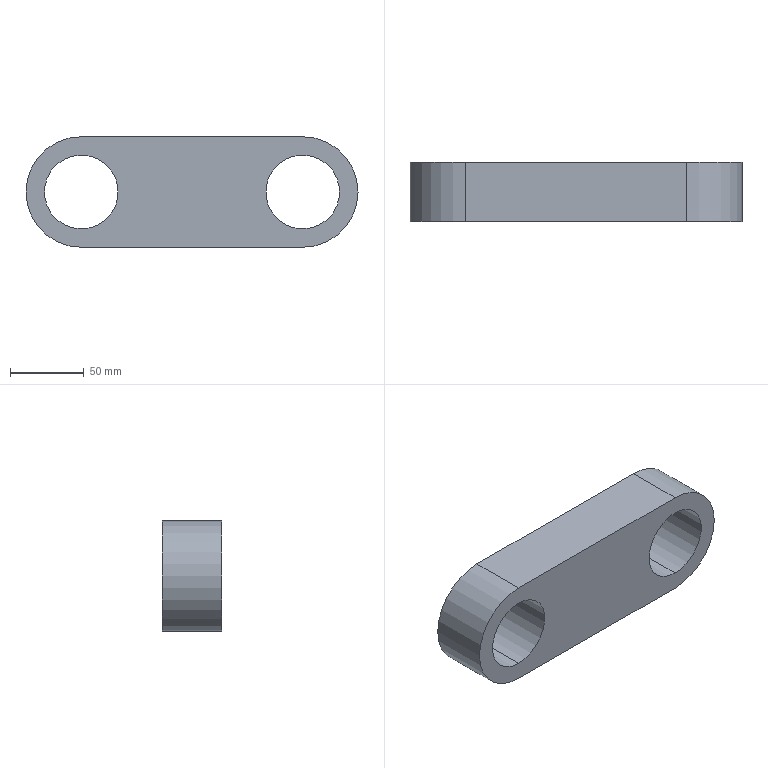Part | STEP file | LM-05-1240_default | 1 solid | 10 faces | box 225 x 40 x 75 mm | volume 469635 mm3 | cylinder 6 | plane 4 | commonest cylinder face diameters 50 x4 75 x2
STEP:
#1=CARTESIAN_POINT('',(0.,0.,0.));
#2=DIRECTION('',(0.,0.,1.));
#3=DIRECTION('',(1.,0.,0.));
#4=AXIS2_PLACEMENT_3D('',#1,#2,#3);
#5=CARTESIAN_POINT('',(75.,40.,-25.));
#6=VERTEX_POINT('',#5);
#7=CARTESIAN_POINT('',(75.,0.,-25.));
#8=VERTEX_POINT('',#7);
#9=CARTESIAN_POINT('',(75.,40.,-25.));
#10=DIRECTION('',(0.,-1.,0.));
#11=VECTOR('',#10,1.);
#12=LINE('',#9,#11);
#13=CARTESIAN_POINT('',(75.,40.,0.));
#14=DIRECTION('',(0.,-1.,0.));
#15=DIRECTION('',(0.,0.,-1.));
#16=AXIS2_PLACEMENT_3D('',#13,#14,#15);
#17=CYLINDRICAL_SURFACE('',#16,25.);
#18=CARTESIAN_POINT('',(6.283,0.));
#19=DIRECTION('',(0.,1.));
#20=VECTOR('',#19,1.);
#21=LINE('',#18,#20);
#22=(GEOMETRIC_REPRESENTATION_CONTEXT(2)PARAMETRIC_REPRESENTATION_CONTEXT()REPRESENTATION_CONTEXT('',''));
#23=DEFINITIONAL_REPRESENTATION('',(#21),#22);
#24=PCURVE('',#17,#23);
#25=CARTESIAN_POINT('',(75.,40.,0.));
#26=DIRECTION('',(0.,-1.,0.));
#27=DIRECTION('',(0.,0.,-1.));
#28=AXIS2_PLACEMENT_3D('',#25,#26,#27);
#29=CYLINDRICAL_SURFACE('',#28,25.);
#30=CARTESIAN_POINT('',(0.,0.));
#31=DIRECTION('',(0.,1.));
#32=VECTOR('',#31,1.);
#33=LINE('',#30,#32);
#34=(GEOMETRIC_REPRESENTATION_CONTEXT(2)PARAMETRIC_REPRESENTATION_CONTEXT()REPRESENTATION_CONTEXT('',''));
#35=DEFINITIONAL_REPRESENTATION('',(#33),#34);
#36=PCURVE('',#29,#35);
#37=SURFACE_CURVE('',#12,(#24,#36),.PCURVE_S1.);
#38=EDGE_CURVE('',#6,#8,#37,.T.);
#39=ORIENTED_EDGE('',*,*,#38,.T.);
#40=CARTESIAN_POINT('',(75.,0.,25.));
#41=VERTEX_POINT('',#40);
#42=CARTESIAN_POINT('',(75.,0.,0.));
#43=DIRECTION('',(0.,-1.,0.));
#44=DIRECTION('',(0.,0.,1.));
#45=AXIS2_PLACEMENT_3D('',#42,#43,#44);
#46=CIRCLE('',#45,25.);
#47=CARTESIAN_POINT('',(3.142,40.));
#48=DIRECTION('',(1.,0.));
#49=VECTOR('',#48,1.);
#50=LINE('',#47,#49);
#51=(GEOMETRIC_REPRESENTATION_CONTEXT(2)PARAMETRIC_REPRESENTATION_CONTEXT()REPRESENTATION_CONTEXT('',''));
#52=DEFINITIONAL_REPRESENTATION('',(#50),#51);
#53=PCURVE('',#17,#52);
#54=CARTESIAN_POINT('',(75.,0.,0.));
#55=DIRECTION('',(0.,-1.,0.));
#56=DIRECTION('',(0.,0.,-1.));
#57=AXIS2_PLACEMENT_3D('',#54,#55,#56);
#58=PLANE('',#57);
#59=CARTESIAN_POINT('',(0.,0.));
#60=DIRECTION('',(-1.,0.));
#61=AXIS2_PLACEMENT_2D('',#59,#60);
#62=CIRCLE('',#61,25.);
#63=(GEOMETRIC_REPRESENTATION_CONTEXT(2)PARAMETRIC_REPRESENTATION_CONTEXT()REPRESENTATION_CONTEXT('',''));
#64=DEFINITIONAL_REPRESENTATION('',(#62),#63);
#65=PCURVE('',#58,#64);
#66=SURFACE_CURVE('',#46,(#53,#65),.PCURVE_S1.);
#67=EDGE_CURVE('',#41,#8,#66,.T.);
#68=ORIENTED_EDGE('',*,*,#67,.F.);
#69=CARTESIAN_POINT('',(75.,40.,25.));
#70=VERTEX_POINT('',#69);
#71=CARTESIAN_POINT('',(75.,40.,25.));
#72=DIRECTION('',(0.,-1.,0.));
#73=VECTOR('',#72,1.);
#74=LINE('',#71,#73);
#75=CARTESIAN_POINT('',(3.142,0.));
#76=DIRECTION('',(0.,1.));
#77=VECTOR('',#76,1.);
#78=LINE('',#75,#77);
#79=(GEOMETRIC_REPRESENTATION_CONTEXT(2)PARAMETRIC_REPRESENTATION_CONTEXT()REPRESENTATION_CONTEXT('',''));
#80=DEFINITIONAL_REPRESENTATION('',(#78),#79);
#81=PCURVE('',#17,#80);
#82=CARTESIAN_POINT('',(3.142,0.));
#83=DIRECTION('',(0.,1.));
#84=VECTOR('',#83,1.);
#85=LINE('',#82,#84);
#86=(GEOMETRIC_REPRESENTATION_CONTEXT(2)PARAMETRIC_REPRESENTATION_CONTEXT()REPRESENTATION_CONTEXT('',''));
#87=DEFINITIONAL_REPRESENTATION('',(#85),#86);
#88=PCURVE('',#29,#87);
#89=SURFACE_CURVE('',#74,(#81,#88),.PCURVE_S1.);
#90=EDGE_CURVE('',#70,#41,#89,.T.);
#91=ORIENTED_EDGE('',*,*,#90,.F.);
#92=CARTESIAN_POINT('',(75.,40.,0.));
#93=DIRECTION('',(0.,-1.,0.));
#94=DIRECTION('',(0.,0.,1.));
#95=AXIS2_PLACEMENT_3D('',#92,#93,#94);
#96=CIRCLE('',#95,25.);
#97=CARTESIAN_POINT('',(3.142,0.));
#98=DIRECTION('',(1.,0.));
#99=VECTOR('',#98,1.);
#100=LINE('',#97,#99);
#101=(GEOMETRIC_REPRESENTATION_CONTEXT(2)PARAMETRIC_REPRESENTATION_CONTEXT()REPRESENTATION_CONTEXT('',''));
#102=DEFINITIONAL_REPRESENTATION('',(#100),#101);
#103=PCURVE('',#17,#102);
#104=CARTESIAN_POINT('',(75.,40.,0.));
#105=DIRECTION('',(0.,-1.,0.));
#106=DIRECTION('',(0.,0.,-1.));
#107=AXIS2_PLACEMENT_3D('',#104,#105,#106);
#108=PLANE('',#107);
#109=CARTESIAN_POINT('',(0.,0.));
#110=DIRECTION('',(-1.,0.));
#111=AXIS2_PLACEMENT_2D('',#109,#110);
#112=CIRCLE('',#111,25.);
#113=(GEOMETRIC_REPRESENTATION_CONTEXT(2)PARAMETRIC_REPRESENTATION_CONTEXT()REPRESENTATION_CONTEXT('',''));
#114=DEFINITIONAL_REPRESENTATION('',(#112),#113);
#115=PCURVE('',#108,#114);
#116=SURFACE_CURVE('',#96,(#103,#115),.PCURVE_S1.);
#117=EDGE_CURVE('',#70,#6,#116,.T.);
#118=ORIENTED_EDGE('',*,*,#117,.T.);
#119=EDGE_LOOP('',(#39,#68,#91,#118));
#120=FACE_BOUND('',#119,.F.);
#121=ADVANCED_FACE('',(#120),#17,.F.);
#122=CARTESIAN_POINT('',(-75.,40.,-25.));
#123=VERTEX_POINT('',#122);
#124=CARTESIAN_POINT('',(-75.,0.,-25.));
#125=VERTEX_POINT('',#124);
#126=CARTESIAN_POINT('',(-75.,40.,-25.));
#127=DIRECTION('',(0.,-1.,0.));
#128=VECTOR('',#127,1.);
#129=LINE('',#126,#128);
#130=CARTESIAN_POINT('',(-75.,40.,0.));
#131=DIRECTION('',(0.,-1.,0.));
#132=DIRECTION('',(0.,0.,-1.));
#133=AXIS2_PLACEMENT_3D('',#130,#131,#132);
#134=CYLINDRICAL_SURFACE('',#133,25.);
#135=CARTESIAN_POINT('',(6.283,0.));
#136=DIRECTION('',(0.,1.));
#137=VECTOR('',#136,1.);
#138=LINE('',#135,#137);
#139=(GEOMETRIC_REPRESENTATION_CONTEXT(2)PARAMETRIC_REPRESENTATION_CONTEXT()REPRESENTATION_CONTEXT('',''));
#140=DEFINITIONAL_REPRESENTATION('',(#138),#139);
#141=PCURVE('',#134,#140);
#142=CARTESIAN_POINT('',(-75.,40.,0.));
#143=DIRECTION('',(0.,-1.,0.));
#144=DIRECTION('',(0.,0.,-1.));
#145=AXIS2_PLACEMENT_3D('',#142,#143,#144);
#146=CYLINDRICAL_SURFACE('',#145,25.);
#147=CARTESIAN_POINT('',(0.,0.));
#148=DIRECTION('',(0.,1.));
#149=VECTOR('',#148,1.);
#150=LINE('',#147,#149);
#151=(GEOMETRIC_REPRESENTATION_CONTEXT(2)PARAMETRIC_REPRESENTATION_CONTEXT()REPRESENTATION_CONTEXT('',''));
#152=DEFINITIONAL_REPRESENTATION('',(#150),#151);
#153=PCURVE('',#146,#152);
#154=SURFACE_CURVE('',#129,(#141,#153),.PCURVE_S1.);
#155=EDGE_CURVE('',#123,#125,#154,.T.);
#156=ORIENTED_EDGE('',*,*,#155,.T.);
#157=CARTESIAN_POINT('',(-75.,0.,25.));
#158=VERTEX_POINT('',#157);
#159=CARTESIAN_POINT('',(-75.,0.,0.));
#160=DIRECTION('',(0.,-1.,0.));
#161=DIRECTION('',(0.,0.,1.));
#162=AXIS2_PLACEMENT_3D('',#159,#160,#161);
#163=CIRCLE('',#162,25.);
#164=CARTESIAN_POINT('',(3.142,40.));
#165=DIRECTION('',(1.,0.));
#166=VECTOR('',#165,1.);
#167=LINE('',#164,#166);
#168=(GEOMETRIC_REPRESENTATION_CONTEXT(2)PARAMETRIC_REPRESENTATION_CONTEXT()REPRESENTATION_CONTEXT('',''));
#169=DEFINITIONAL_REPRESENTATION('',(#167),#168);
#170=PCURVE('',#134,#169);
#171=CARTESIAN_POINT('',(0.,-150.));
#172=DIRECTION('',(-1.,0.));
#173=AXIS2_PLACEMENT_2D('',#171,#172);
#174=CIRCLE('',#173,25.);
#175=(GEOMETRIC_REPRESENTATION_CONTEXT(2)PARAMETRIC_REPRESENTATION_CONTEXT()REPRESENTATION_CONTEXT('',''));
#176=DEFINITIONAL_REPRESENTATION('',(#174),#175);
#177=PCURVE('',#58,#176);
#178=SURFACE_CURVE('',#163,(#170,#177),.PCURVE_S1.);
#179=EDGE_CURVE('',#158,#125,#178,.T.);
#180=ORIENTED_EDGE('',*,*,#179,.F.);
#181=CARTESIAN_POINT('',(-75.,40.,25.));
#182=VERTEX_POINT('',#181);
#183=CARTESIAN_POINT('',(-75.,40.,25.));
#184=DIRECTION('',(0.,-1.,0.));
#185=VECTOR('',#184,1.);
#186=LINE('',#183,#185);
#187=CARTESIAN_POINT('',(3.142,0.));
#188=DIRECTION('',(0.,1.));
#189=VECTOR('',#188,1.);
#190=LINE('',#187,#189);
#191=(GEOMETRIC_REPRESENTATION_CONTEXT(2)PARAMETRIC_REPRESENTATION_CONTEXT()REPRESENTATION_CONTEXT('',''));
#192=DEFINITIONAL_REPRESENTATION('',(#190),#191);
#193=PCURVE('',#134,#192);
#194=CARTESIAN_POINT('',(3.142,0.));
#195=DIRECTION('',(0.,1.));
#196=VECTOR('',#195,1.);
#197=LINE('',#194,#196);
#198=(GEOMETRIC_REPRESENTATION_CONTEXT(2)PARAMETRIC_REPRESENTATION_CONTEXT()REPRESENTATION_CONTEXT('',''));
#199=DEFINITIONAL_REPRESENTATION('',(#197),#198);
#200=PCURVE('',#146,#199);
#201=SURFACE_CURVE('',#186,(#193,#200),.PCURVE_S1.);
#202=EDGE_CURVE('',#182,#158,#201,.T.);
#203=ORIENTED_EDGE('',*,*,#202,.F.);
#204=CARTESIAN_POINT('',(-75.,40.,0.));
#205=DIRECTION('',(0.,-1.,0.));
#206=DIRECTION('',(0.,0.,1.));
#207=AXIS2_PLACEMENT_3D('',#204,#205,#206);
#208=CIRCLE('',#207,25.);
#209=CARTESIAN_POINT('',(3.142,0.));
#210=DIRECTION('',(1.,0.));
#211=VECTOR('',#210,1.);
#212=LINE('',#209,#211);
#213=(GEOMETRIC_REPRESENTATION_CONTEXT(2)PARAMETRIC_REPRESENTATION_CONTEXT()REPRESENTATION_CONTEXT('',''));
#214=DEFINITIONAL_REPRESENTATION('',(#212),#213);
#215=PCURVE('',#134,#214);
#216=CARTESIAN_POINT('',(0.,-150.));
#217=DIRECTION('',(-1.,0.));
#218=AXIS2_PLACEMENT_2D('',#216,#217);
#219=CIRCLE('',#218,25.);
#220=(GEOMETRIC_REPRESENTATION_CONTEXT(2)PARAMETRIC_REPRESENTATION_CONTEXT()REPRESENTATION_CONTEXT('',''));
#221=DEFINITIONAL_REPRESENTATION('',(#219),#220);
#222=PCURVE('',#108,#221);
#223=SURFACE_CURVE('',#208,(#215,#222),.PCURVE_S1.);
#224=EDGE_CURVE('',#182,#123,#223,.T.);
#225=ORIENTED_EDGE('',*,*,#224,.T.);
#226=EDGE_LOOP('',(#156,#180,#203,#225));
#227=FACE_BOUND('',#226,.F.);
#228=ADVANCED_FACE('',(#227),#134,.F.);
#229=CARTESIAN_POINT('',(75.,0.,-37.5));
#230=VERTEX_POINT('',#229);
#231=CARTESIAN_POINT('',(75.,0.,37.5));
#232=VERTEX_POINT('',#231);
#233=CARTESIAN_POINT('',(75.,0.,0.));
#234=DIRECTION('',(0.,-1.,0.));
#235=DIRECTION('',(0.,0.,-1.));
#236=AXIS2_PLACEMENT_3D('',#233,#234,#235);
#237=CIRCLE('',#236,37.5);
#238=CARTESIAN_POINT('',(75.,40.,0.));
#239=DIRECTION('',(0.,-1.,0.));
#240=DIRECTION('',(0.,0.,-1.));
#241=AXIS2_PLACEMENT_3D('',#238,#239,#240);
#242=CYLINDRICAL_SURFACE('',#241,37.5);
#243=CARTESIAN_POINT('',(0.,40.));
#244=DIRECTION('',(1.,0.));
#245=VECTOR('',#244,1.);
#246=LINE('',#243,#245);
#247=(GEOMETRIC_REPRESENTATION_CONTEXT(2)PARAMETRIC_REPRESENTATION_CONTEXT()REPRESENTATION_CONTEXT('',''));
#248=DEFINITIONAL_REPRESENTATION('',(#246),#247);
#249=PCURVE('',#242,#248);
#250=CARTESIAN_POINT('',(0.,0.));
#251=DIRECTION('',(1.,0.));
#252=AXIS2_PLACEMENT_2D('',#250,#251);
#253=CIRCLE('',#252,37.5);
#254=(GEOMETRIC_REPRESENTATION_CONTEXT(2)PARAMETRIC_REPRESENTATION_CONTEXT()REPRESENTATION_CONTEXT('',''));
#255=DEFINITIONAL_REPRESENTATION('',(#253),#254);
#256=PCURVE('',#58,#255);
#257=SURFACE_CURVE('',#237,(#249,#256),.PCURVE_S1.);
#258=EDGE_CURVE('',#230,#232,#257,.T.);
#259=ORIENTED_EDGE('',*,*,#258,.F.);
#260=CARTESIAN_POINT('',(75.,40.,-37.5));
#261=VERTEX_POINT('',#260);
#262=CARTESIAN_POINT('',(75.,40.,-37.5));
#263=DIRECTION('',(0.,-1.,0.));
#264=VECTOR('',#263,1.);
#265=LINE('',#262,#264);
#266=CARTESIAN_POINT('',(0.,0.));
#267=DIRECTION('',(0.,1.));
#268=VECTOR('',#267,1.);
#269=LINE('',#266,#268);
#270=(GEOMETRIC_REPRESENTATION_CONTEXT(2)PARAMETRIC_REPRESENTATION_CONTEXT()REPRESENTATION_CONTEXT('',''));
#271=DEFINITIONAL_REPRESENTATION('',(#269),#270);
#272=PCURVE('',#242,#271);
#273=CARTESIAN_POINT('',(-75.,40.,-37.5));
#274=DIRECTION('',(0.,0.,-1.));
#275=DIRECTION('',(-1.,0.,0.));
#276=AXIS2_PLACEMENT_3D('',#273,#274,#275);
#277=PLANE('',#276);
#278=CARTESIAN_POINT('',(-150.,0.));
#279=DIRECTION('',(0.,-1.));
#280=VECTOR('',#279,1.);
#281=LINE('',#278,#280);
#282=(GEOMETRIC_REPRESENTATION_CONTEXT(2)PARAMETRIC_REPRESENTATION_CONTEXT()REPRESENTATION_CONTEXT('',''));
#283=DEFINITIONAL_REPRESENTATION('',(#281),#282);
#284=PCURVE('',#277,#283);
#285=SURFACE_CURVE('',#265,(#272,#284),.PCURVE_S1.);
#286=EDGE_CURVE('',#261,#230,#285,.T.);
#287=ORIENTED_EDGE('',*,*,#286,.F.);
#288=CARTESIAN_POINT('',(75.,40.,37.5));
#289=VERTEX_POINT('',#288);
#290=CARTESIAN_POINT('',(75.,40.,0.));
#291=DIRECTION('',(0.,-1.,0.));
#292=DIRECTION('',(0.,0.,-1.));
#293=AXIS2_PLACEMENT_3D('',#290,#291,#292);
#294=CIRCLE('',#293,37.5);
#295=CARTESIAN_POINT('',(0.,0.));
#296=DIRECTION('',(1.,0.));
#297=VECTOR('',#296,1.);
#298=LINE('',#295,#297);
#299=(GEOMETRIC_REPRESENTATION_CONTEXT(2)PARAMETRIC_REPRESENTATION_CONTEXT()REPRESENTATION_CONTEXT('',''));
#300=DEFINITIONAL_REPRESENTATION('',(#298),#299);
#301=PCURVE('',#242,#300);
#302=CARTESIAN_POINT('',(0.,0.));
#303=DIRECTION('',(1.,0.));
#304=AXIS2_PLACEMENT_2D('',#302,#303);
#305=CIRCLE('',#304,37.5);
#306=(GEOMETRIC_REPRESENTATION_CONTEXT(2)PARAMETRIC_REPRESENTATION_CONTEXT()REPRESENTATION_CONTEXT('',''));
#307=DEFINITIONAL_REPRESENTATION('',(#305),#306);
#308=PCURVE('',#108,#307);
#309=SURFACE_CURVE('',#294,(#301,#308),.PCURVE_S1.);
#310=EDGE_CURVE('',#261,#289,#309,.T.);
#311=ORIENTED_EDGE('',*,*,#310,.T.);
#312=CARTESIAN_POINT('',(75.,40.,37.5));
#313=DIRECTION('',(0.,-1.,0.));
#314=VECTOR('',#313,1.);
#315=LINE('',#312,#314);
#316=CARTESIAN_POINT('',(3.142,0.));
#317=DIRECTION('',(0.,1.));
#318=VECTOR('',#317,1.);
#319=LINE('',#316,#318);
#320=(GEOMETRIC_REPRESENTATION_CONTEXT(2)PARAMETRIC_REPRESENTATION_CONTEXT()REPRESENTATION_CONTEXT('',''));
#321=DEFINITIONAL_REPRESENTATION('',(#319),#320);
#322=PCURVE('',#242,#321);
#323=CARTESIAN_POINT('',(75.,40.,37.5));
#324=DIRECTION('',(0.,0.,1.));
#325=DIRECTION('',(1.,0.,0.));
#326=AXIS2_PLACEMENT_3D('',#323,#324,#325);
#327=PLANE('',#326);
#328=CARTESIAN_POINT('',(0.,0.));
#329=DIRECTION('',(0.,-1.));
#330=VECTOR('',#329,1.);
#331=LINE('',#328,#330);
#332=(GEOMETRIC_REPRESENTATION_CONTEXT(2)PARAMETRIC_REPRESENTATION_CONTEXT()REPRESENTATION_CONTEXT('',''));
#333=DEFINITIONAL_REPRESENTATION('',(#331),#332);
#334=PCURVE('',#327,#333);
#335=SURFACE_CURVE('',#315,(#322,#334),.PCURVE_S1.);
#336=EDGE_CURVE('',#289,#232,#335,.T.);
#337=ORIENTED_EDGE('',*,*,#336,.T.);
#338=EDGE_LOOP('',(#259,#287,#311,#337));
#339=FACE_BOUND('',#338,.T.);
#340=ADVANCED_FACE('',(#339),#242,.T.);
#341=CARTESIAN_POINT('',(-75.,0.,-37.5));
#342=VERTEX_POINT('',#341);
#343=CARTESIAN_POINT('',(-75.,0.,-37.5));
#344=DIRECTION('',(1.,0.,0.));
#345=VECTOR('',#344,1.);
#346=LINE('',#343,#345);
#347=CARTESIAN_POINT('',(0.,-40.));
#348=DIRECTION('',(-1.,0.));
#349=VECTOR('',#348,1.);
#350=LINE('',#347,#349);
#351=(GEOMETRIC_REPRESENTATION_CONTEXT(2)PARAMETRIC_REPRESENTATION_CONTEXT()REPRESENTATION_CONTEXT('',''));
#352=DEFINITIONAL_REPRESENTATION('',(#350),#351);
#353=PCURVE('',#277,#352);
#354=CARTESIAN_POINT('',(37.5,-150.));
#355=DIRECTION('',(0.,1.));
#356=VECTOR('',#355,1.);
#357=LINE('',#354,#356);
#358=(GEOMETRIC_REPRESENTATION_CONTEXT(2)PARAMETRIC_REPRESENTATION_CONTEXT()REPRESENTATION_CONTEXT('',''));
#359=DEFINITIONAL_REPRESENTATION('',(#357),#358);
#360=PCURVE('',#58,#359);
#361=SURFACE_CURVE('',#346,(#353,#360),.PCURVE_S1.);
#362=EDGE_CURVE('',#342,#230,#361,.T.);
#363=ORIENTED_EDGE('',*,*,#362,.F.);
#364=CARTESIAN_POINT('',(-75.,40.,-37.5));
#365=VERTEX_POINT('',#364);
#366=CARTESIAN_POINT('',(-75.,40.,-37.5));
#367=DIRECTION('',(0.,-1.,0.));
#368=VECTOR('',#367,1.);
#369=LINE('',#366,#368);
#370=CARTESIAN_POINT('',(0.,0.));
#371=DIRECTION('',(0.,-1.));
#372=VECTOR('',#371,1.);
#373=LINE('',#370,#372);
#374=(GEOMETRIC_REPRESENTATION_CONTEXT(2)PARAMETRIC_REPRESENTATION_CONTEXT()REPRESENTATION_CONTEXT('',''));
#375=DEFINITIONAL_REPRESENTATION('',(#373),#374);
#376=PCURVE('',#277,#375);
#377=CARTESIAN_POINT('',(-75.,40.,0.));
#378=DIRECTION('',(0.,-1.,0.));
#379=DIRECTION('',(0.,0.,-1.));
#380=AXIS2_PLACEMENT_3D('',#377,#378,#379);
#381=CYLINDRICAL_SURFACE('',#380,37.5);
#382=CARTESIAN_POINT('',(6.283,0.));
#383=DIRECTION('',(0.,1.));
#384=VECTOR('',#383,1.);
#385=LINE('',#382,#384);
#386=(GEOMETRIC_REPRESENTATION_CONTEXT(2)PARAMETRIC_REPRESENTATION_CONTEXT()REPRESENTATION_CONTEXT('',''));
#387=DEFINITIONAL_REPRESENTATION('',(#385),#386);
#388=PCURVE('',#381,#387);
#389=SURFACE_CURVE('',#369,(#376,#388),.PCURVE_S1.);
#390=EDGE_CURVE('',#365,#342,#389,.T.);
#391=ORIENTED_EDGE('',*,*,#390,.F.);
#392=CARTESIAN_POINT('',(-75.,40.,-37.5));
#393=DIRECTION('',(1.,0.,0.));
#394=VECTOR('',#393,1.);
#395=LINE('',#392,#394);
#396=CARTESIAN_POINT('',(0.,0.));
#397=DIRECTION('',(-1.,0.));
#398=VECTOR('',#397,1.);
#399=LINE('',#396,#398);
#400=(GEOMETRIC_REPRESENTATION_CONTEXT(2)PARAMETRIC_REPRESENTATION_CONTEXT()REPRESENTATION_CONTEXT('',''));
#401=DEFINITIONAL_REPRESENTATION('',(#399),#400);
#402=PCURVE('',#277,#401);
#403=CARTESIAN_POINT('',(37.5,-150.));
#404=DIRECTION('',(0.,1.));
#405=VECTOR('',#404,1.);
#406=LINE('',#403,#405);
#407=(GEOMETRIC_REPRESENTATION_CONTEXT(2)PARAMETRIC_REPRESENTATION_CONTEXT()REPRESENTATION_CONTEXT('',''));
#408=DEFINITIONAL_REPRESENTATION('',(#406),#407);
#409=PCURVE('',#108,#408);
#410=SURFACE_CURVE('',#395,(#402,#409),.PCURVE_S1.);
#411=EDGE_CURVE('',#365,#261,#410,.T.);
#412=ORIENTED_EDGE('',*,*,#411,.T.);
#413=ORIENTED_EDGE('',*,*,#286,.T.);
#414=EDGE_LOOP('',(#363,#391,#412,#413));
#415=FACE_BOUND('',#414,.T.);
#416=ADVANCED_FACE('',(#415),#277,.T.);
#417=CARTESIAN_POINT('',(-75.,0.,37.5));
#418=VERTEX_POINT('',#417);
#419=CARTESIAN_POINT('',(-75.,0.,0.));
#420=DIRECTION('',(0.,-1.,0.));
#421=DIRECTION('',(0.,0.,-1.));
#422=AXIS2_PLACEMENT_3D('',#419,#420,#421);
#423=CIRCLE('',#422,37.5);
#424=CARTESIAN_POINT('',(0.,40.));
#425=DIRECTION('',(1.,0.));
#426=VECTOR('',#425,1.);
#427=LINE('',#424,#426);
#428=(GEOMETRIC_REPRESENTATION_CONTEXT(2)PARAMETRIC_REPRESENTATION_CONTEXT()REPRESENTATION_CONTEXT('',''));
#429=DEFINITIONAL_REPRESENTATION('',(#427),#428);
#430=PCURVE('',#381,#429);
#431=CARTESIAN_POINT('',(0.,-150.));
#432=DIRECTION('',(1.,0.));
#433=AXIS2_PLACEMENT_2D('',#431,#432);
#434=CIRCLE('',#433,37.5);
#435=(GEOMETRIC_REPRESENTATION_CONTEXT(2)PARAMETRIC_REPRESENTATION_CONTEXT()REPRESENTATION_CONTEXT('',''));
#436=DEFINITIONAL_REPRESENTATION('',(#434),#435);
#437=PCURVE('',#58,#436);
#438=SURFACE_CURVE('',#423,(#430,#437),.PCURVE_S1.);
#439=EDGE_CURVE('',#418,#342,#438,.T.);
#440=ORIENTED_EDGE('',*,*,#439,.F.);
#441=CARTESIAN_POINT('',(-75.,40.,37.5));
#442=VERTEX_POINT('',#441);
#443=CARTESIAN_POINT('',(-75.,40.,37.5));
#444=DIRECTION('',(0.,-1.,0.));
#445=VECTOR('',#444,1.);
#446=LINE('',#443,#445);
#447=CARTESIAN_POINT('',(3.142,0.));
#448=DIRECTION('',(0.,1.));
#449=VECTOR('',#448,1.);
#450=LINE('',#447,#449);
#451=(GEOMETRIC_REPRESENTATION_CONTEXT(2)PARAMETRIC_REPRESENTATION_CONTEXT()REPRESENTATION_CONTEXT('',''));
#452=DEFINITIONAL_REPRESENTATION('',(#450),#451);
#453=PCURVE('',#381,#452);
#454=CARTESIAN_POINT('',(-150.,0.));
#455=DIRECTION('',(0.,-1.));
#456=VECTOR('',#455,1.);
#457=LINE('',#454,#456);
#458=(GEOMETRIC_REPRESENTATION_CONTEXT(2)PARAMETRIC_REPRESENTATION_CONTEXT()REPRESENTATION_CONTEXT('',''));
#459=DEFINITIONAL_REPRESENTATION('',(#457),#458);
#460=PCURVE('',#327,#459);
#461=SURFACE_CURVE('',#446,(#453,#460),.PCURVE_S1.);
#462=EDGE_CURVE('',#442,#418,#461,.T.);
#463=ORIENTED_EDGE('',*,*,#462,.F.);
#464=CARTESIAN_POINT('',(-75.,40.,0.));
#465=DIRECTION('',(0.,-1.,0.));
#466=DIRECTION('',(0.,0.,-1.));
#467=AXIS2_PLACEMENT_3D('',#464,#465,#466);
#468=CIRCLE('',#467,37.5);
#469=CARTESIAN_POINT('',(0.,0.));
#470=DIRECTION('',(1.,0.));
#471=VECTOR('',#470,1.);
#472=LINE('',#469,#471);
#473=(GEOMETRIC_REPRESENTATION_CONTEXT(2)PARAMETRIC_REPRESENTATION_CONTEXT()REPRESENTATION_CONTEXT('',''));
#474=DEFINITIONAL_REPRESENTATION('',(#472),#473);
#475=PCURVE('',#381,#474);
#476=CARTESIAN_POINT('',(0.,-150.));
#477=DIRECTION('',(1.,0.));
#478=AXIS2_PLACEMENT_2D('',#476,#477);
#479=CIRCLE('',#478,37.5);
#480=(GEOMETRIC_REPRESENTATION_CONTEXT(2)PARAMETRIC_REPRESENTATION_CONTEXT()REPRESENTATION_CONTEXT('',''));
#481=DEFINITIONAL_REPRESENTATION('',(#479),#480);
#482=PCURVE('',#108,#481);
#483=SURFACE_CURVE('',#468,(#475,#482),.PCURVE_S1.);
#484=EDGE_CURVE('',#442,#365,#483,.T.);
#485=ORIENTED_EDGE('',*,*,#484,.T.);
#486=ORIENTED_EDGE('',*,*,#390,.T.);
#487=EDGE_LOOP('',(#440,#463,#485,#486));
#488=FACE_BOUND('',#487,.T.);
#489=ADVANCED_FACE('',(#488),#381,.T.);
#490=CARTESIAN_POINT('',(75.,0.,37.5));
#491=DIRECTION('',(-1.,0.,0.));
#492=VECTOR('',#491,1.);
#493=LINE('',#490,#492);
#494=CARTESIAN_POINT('',(0.,-40.));
#495=DIRECTION('',(-1.,0.));
#496=VECTOR('',#495,1.);
#497=LINE('',#494,#496);
#498=(GEOMETRIC_REPRESENTATION_CONTEXT(2)PARAMETRIC_REPRESENTATION_CONTEXT()REPRESENTATION_CONTEXT('',''));
#499=DEFINITIONAL_REPRESENTATION('',(#497),#498);
#500=PCURVE('',#327,#499);
#501=CARTESIAN_POINT('',(-37.5,0.));
#502=DIRECTION('',(0.,-1.));
#503=VECTOR('',#502,1.);
#504=LINE('',#501,#503);
#505=(GEOMETRIC_REPRESENTATION_CONTEXT(2)PARAMETRIC_REPRESENTATION_CONTEXT()REPRESENTATION_CONTEXT('',''));
#506=DEFINITIONAL_REPRESENTATION('',(#504),#505);
#507=PCURVE('',#58,#506);
#508=SURFACE_CURVE('',#493,(#500,#507),.PCURVE_S1.);
#509=EDGE_CURVE('',#232,#418,#508,.T.);
#510=ORIENTED_EDGE('',*,*,#509,.F.);
#511=ORIENTED_EDGE('',*,*,#336,.F.);
#512=CARTESIAN_POINT('',(75.,40.,37.5));
#513=DIRECTION('',(-1.,0.,0.));
#514=VECTOR('',#513,1.);
#515=LINE('',#512,#514);
#516=CARTESIAN_POINT('',(0.,0.));
#517=DIRECTION('',(-1.,0.));
#518=VECTOR('',#517,1.);
#519=LINE('',#516,#518);
#520=(GEOMETRIC_REPRESENTATION_CONTEXT(2)PARAMETRIC_REPRESENTATION_CONTEXT()REPRESENTATION_CONTEXT('',''));
#521=DEFINITIONAL_REPRESENTATION('',(#519),#520);
#522=PCURVE('',#327,#521);
#523=CARTESIAN_POINT('',(-37.5,0.));
#524=DIRECTION('',(0.,-1.));
#525=VECTOR('',#524,1.);
#526=LINE('',#523,#525);
#527=(GEOMETRIC_REPRESENTATION_CONTEXT(2)PARAMETRIC_REPRESENTATION_CONTEXT()REPRESENTATION_CONTEXT('',''));
#528=DEFINITIONAL_REPRESENTATION('',(#526),#527);
#529=PCURVE('',#108,#528);
#530=SURFACE_CURVE('',#515,(#522,#529),.PCURVE_S1.);
#531=EDGE_CURVE('',#289,#442,#530,.T.);
#532=ORIENTED_EDGE('',*,*,#531,.T.);
#533=ORIENTED_EDGE('',*,*,#462,.T.);
#534=EDGE_LOOP('',(#510,#511,#532,#533));
#535=FACE_BOUND('',#534,.T.);
#536=ADVANCED_FACE('',(#535),#327,.T.);
#537=CARTESIAN_POINT('',(75.,40.,0.));
#538=DIRECTION('',(0.,-1.,0.));
#539=DIRECTION('',(0.,0.,1.));
#540=AXIS2_PLACEMENT_3D('',#537,#538,#539);
#541=CIRCLE('',#540,25.);
#542=CARTESIAN_POINT('',(0.,0.));
#543=DIRECTION('',(-1.,0.));
#544=AXIS2_PLACEMENT_2D('',#542,#543);
#545=CIRCLE('',#544,25.);
#546=(GEOMETRIC_REPRESENTATION_CONTEXT(2)PARAMETRIC_REPRESENTATION_CONTEXT()REPRESENTATION_CONTEXT('',''));
#547=DEFINITIONAL_REPRESENTATION('',(#545),#546);
#548=PCURVE('',#108,#547);
#549=CARTESIAN_POINT('',(-3.142,0.));
#550=DIRECTION('',(1.,0.));
#551=VECTOR('',#550,1.);
#552=LINE('',#549,#551);
#553=(GEOMETRIC_REPRESENTATION_CONTEXT(2)PARAMETRIC_REPRESENTATION_CONTEXT()REPRESENTATION_CONTEXT('',''));
#554=DEFINITIONAL_REPRESENTATION('',(#552),#553);
#555=PCURVE('',#29,#554);
#556=SURFACE_CURVE('',#541,(#548,#555),.PCURVE_S1.);
#557=EDGE_CURVE('',#6,#70,#556,.T.);
#558=ORIENTED_EDGE('',*,*,#557,.T.);
#559=ORIENTED_EDGE('',*,*,#117,.T.);
#560=EDGE_LOOP('',(#558,#559));
#561=FACE_BOUND('',#560,.T.);
#562=CARTESIAN_POINT('',(-75.,40.,0.));
#563=DIRECTION('',(0.,-1.,0.));
#564=DIRECTION('',(0.,0.,1.));
#565=AXIS2_PLACEMENT_3D('',#562,#563,#564);
#566=CIRCLE('',#565,25.);
#567=CARTESIAN_POINT('',(0.,-150.));
#568=DIRECTION('',(-1.,0.));
#569=AXIS2_PLACEMENT_2D('',#567,#568);
#570=CIRCLE('',#569,25.);
#571=(GEOMETRIC_REPRESENTATION_CONTEXT(2)PARAMETRIC_REPRESENTATION_CONTEXT()REPRESENTATION_CONTEXT('',''));
#572=DEFINITIONAL_REPRESENTATION('',(#570),#571);
#573=PCURVE('',#108,#572);
#574=CARTESIAN_POINT('',(-3.142,0.));
#575=DIRECTION('',(1.,0.));
#576=VECTOR('',#575,1.);
#577=LINE('',#574,#576);
#578=(GEOMETRIC_REPRESENTATION_CONTEXT(2)PARAMETRIC_REPRESENTATION_CONTEXT()REPRESENTATION_CONTEXT('',''));
#579=DEFINITIONAL_REPRESENTATION('',(#577),#578);
#580=PCURVE('',#146,#579);
#581=SURFACE_CURVE('',#566,(#573,#580),.PCURVE_S1.);
#582=EDGE_CURVE('',#123,#182,#581,.T.);
#583=ORIENTED_EDGE('',*,*,#582,.T.);
#584=ORIENTED_EDGE('',*,*,#224,.T.);
#585=EDGE_LOOP('',(#583,#584));
#586=FACE_BOUND('',#585,.T.);
#587=ORIENTED_EDGE('',*,*,#310,.F.);
#588=ORIENTED_EDGE('',*,*,#411,.F.);
#589=ORIENTED_EDGE('',*,*,#484,.F.);
#590=ORIENTED_EDGE('',*,*,#531,.F.);
#591=EDGE_LOOP('',(#587,#588,#589,#590));
#592=FACE_BOUND('',#591,.T.);
#593=ADVANCED_FACE('',(#561,#586,#592),#108,.F.);
#594=CARTESIAN_POINT('',(75.,0.,0.));
#595=DIRECTION('',(0.,-1.,0.));
#596=DIRECTION('',(0.,0.,1.));
#597=AXIS2_PLACEMENT_3D('',#594,#595,#596);
#598=CIRCLE('',#597,25.);
#599=CARTESIAN_POINT('',(0.,0.));
#600=DIRECTION('',(-1.,0.));
#601=AXIS2_PLACEMENT_2D('',#599,#600);
#602=CIRCLE('',#601,25.);
#603=(GEOMETRIC_REPRESENTATION_CONTEXT(2)PARAMETRIC_REPRESENTATION_CONTEXT()REPRESENTATION_CONTEXT('',''));
#604=DEFINITIONAL_REPRESENTATION('',(#602),#603);
#605=PCURVE('',#58,#604);
#606=CARTESIAN_POINT('',(-3.142,40.));
#607=DIRECTION('',(1.,0.));
#608=VECTOR('',#607,1.);
#609=LINE('',#606,#608);
#610=(GEOMETRIC_REPRESENTATION_CONTEXT(2)PARAMETRIC_REPRESENTATION_CONTEXT()REPRESENTATION_CONTEXT('',''));
#611=DEFINITIONAL_REPRESENTATION('',(#609),#610);
#612=PCURVE('',#29,#611);
#613=SURFACE_CURVE('',#598,(#605,#612),.PCURVE_S1.);
#614=EDGE_CURVE('',#8,#41,#613,.T.);
#615=ORIENTED_EDGE('',*,*,#614,.F.);
#616=ORIENTED_EDGE('',*,*,#67,.F.);
#617=EDGE_LOOP('',(#615,#616));
#618=FACE_BOUND('',#617,.T.);
#619=CARTESIAN_POINT('',(-75.,0.,0.));
#620=DIRECTION('',(0.,-1.,0.));
#621=DIRECTION('',(0.,0.,1.));
#622=AXIS2_PLACEMENT_3D('',#619,#620,#621);
#623=CIRCLE('',#622,25.);
#624=CARTESIAN_POINT('',(0.,-150.));
#625=DIRECTION('',(-1.,0.));
#626=AXIS2_PLACEMENT_2D('',#624,#625);
#627=CIRCLE('',#626,25.);
#628=(GEOMETRIC_REPRESENTATION_CONTEXT(2)PARAMETRIC_REPRESENTATION_CONTEXT()REPRESENTATION_CONTEXT('',''));
#629=DEFINITIONAL_REPRESENTATION('',(#627),#628);
#630=PCURVE('',#58,#629);
#631=CARTESIAN_POINT('',(-3.142,40.));
#632=DIRECTION('',(1.,0.));
#633=VECTOR('',#632,1.);
#634=LINE('',#631,#633);
#635=(GEOMETRIC_REPRESENTATION_CONTEXT(2)PARAMETRIC_REPRESENTATION_CONTEXT()REPRESENTATION_CONTEXT('',''));
#636=DEFINITIONAL_REPRESENTATION('',(#634),#635);
#637=PCURVE('',#146,#636);
#638=SURFACE_CURVE('',#623,(#630,#637),.PCURVE_S1.);
#639=EDGE_CURVE('',#125,#158,#638,.T.);
#640=ORIENTED_EDGE('',*,*,#639,.F.);
#641=ORIENTED_EDGE('',*,*,#179,.F.);
#642=EDGE_LOOP('',(#640,#641));
#643=FACE_BOUND('',#642,.T.);
#644=ORIENTED_EDGE('',*,*,#258,.T.);
#645=ORIENTED_EDGE('',*,*,#509,.T.);
#646=ORIENTED_EDGE('',*,*,#439,.T.);
#647=ORIENTED_EDGE('',*,*,#362,.T.);
#648=EDGE_LOOP('',(#644,#645,#646,#647));
#649=FACE_BOUND('',#648,.T.);
#650=ADVANCED_FACE('',(#618,#643,#649),#58,.T.);
#651=ORIENTED_EDGE('',*,*,#639,.F.);
#652=ORIENTED_EDGE('',*,*,#155,.F.);
#653=ORIENTED_EDGE('',*,*,#582,.T.);
#654=ORIENTED_EDGE('',*,*,#202,.T.);
#655=EDGE_LOOP('',(#651,#652,#653,#654));
#656=FACE_BOUND('',#655,.F.);
#657=ADVANCED_FACE('',(#656),#146,.F.);
#658=ORIENTED_EDGE('',*,*,#614,.F.);
#659=ORIENTED_EDGE('',*,*,#38,.F.);
#660=ORIENTED_EDGE('',*,*,#557,.T.);
#661=ORIENTED_EDGE('',*,*,#90,.T.);
#662=EDGE_LOOP('',(#658,#659,#660,#661));
#663=FACE_BOUND('',#662,.F.);
#664=ADVANCED_FACE('',(#663),#29,.F.);
#665=CLOSED_SHELL('',(#121,#228,#340,#416,#489,#536,#593,#650,#657,#664));
#666=MANIFOLD_SOLID_BREP('',#665);
#667=(LENGTH_UNIT()NAMED_UNIT(*)SI_UNIT(.MILLI.,.METRE.));
#668=UNCERTAINTY_MEASURE_WITH_UNIT(LENGTH_MEASURE(0.0000001),#667,'','');
#669=(NAMED_UNIT(*)PLANE_ANGLE_UNIT()SI_UNIT($,.RADIAN.));
#670=(NAMED_UNIT(*)SI_UNIT($,.STERADIAN.)SOLID_ANGLE_UNIT());
#671=(GEOMETRIC_REPRESENTATION_CONTEXT(3)GLOBAL_UNCERTAINTY_ASSIGNED_CONTEXT((#668))GLOBAL_UNIT_ASSIGNED_CONTEXT((#667,#669,#670))REPRESENTATION_CONTEXT('',''));
#672=ADVANCED_BREP_SHAPE_REPRESENTATION('',(#4,#666),#671);